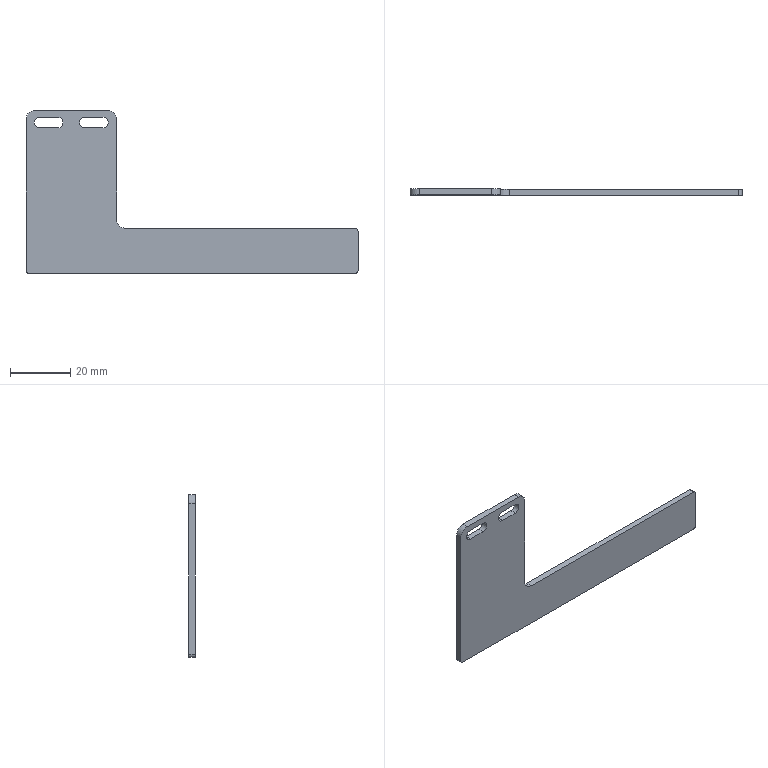Part | NX | features BREP 1 | 1 solid | 22 faces | box 110 x 2 x 54 mm | volume 5512 mm3 | plane 12 | cylinder 10 | commonest cylinder face diameters 3.5 x4 2 x3 6 x3
STEP:
#1=CARTESIAN_POINT('',(-55.,-2.,1.));
#2=VERTEX_POINT('',#1);
#3=CARTESIAN_POINT('',(-54.,-2.,0.));
#4=VERTEX_POINT('',#3);
#5=CARTESIAN_POINT('',(-54.,-2.,1.));
#6=DIRECTION('',(0.,-1.,0.));
#7=DIRECTION('',(-1.,0.,0.));
#8=AXIS2_PLACEMENT_3D('',#5,#6,#7);
#9=CIRCLE('',#8,1.);
#10=EDGE_CURVE('',#2,#4,#9,.T.);
#11=ORIENTED_EDGE('',*,*,#10,.F.);
#12=CARTESIAN_POINT('',(-55.,0.,1.));
#13=VERTEX_POINT('',#12);
#14=CARTESIAN_POINT('',(-55.,-2.,1.));
#15=DIRECTION('',(0.,-1.,0.));
#16=VECTOR('',#15,1000.);
#17=LINE('',#14,#16);
#18=EDGE_CURVE('',#13,#2,#17,.T.);
#19=ORIENTED_EDGE('',*,*,#18,.F.);
#20=CARTESIAN_POINT('',(-54.,0.,0.));
#21=VERTEX_POINT('',#20);
#22=CARTESIAN_POINT('',(-54.,0.,1.));
#23=DIRECTION('',(0.,1.,0.));
#24=DIRECTION('',(-1.,0.,0.));
#25=AXIS2_PLACEMENT_3D('',#22,#23,#24);
#26=CIRCLE('',#25,1.);
#27=EDGE_CURVE('',#21,#13,#26,.T.);
#28=ORIENTED_EDGE('',*,*,#27,.F.);
#29=CARTESIAN_POINT('',(-54.,0.,0.));
#30=DIRECTION('',(0.,1.,0.));
#31=VECTOR('',#30,1000.);
#32=LINE('',#29,#31);
#33=EDGE_CURVE('',#4,#21,#32,.T.);
#34=ORIENTED_EDGE('',*,*,#33,.F.);
#35=EDGE_LOOP('',(#11,#19,#28,#34));
#36=FACE_BOUND('',#35,.T.);
#37=CARTESIAN_POINT('',(-54.,0.,1.));
#38=DIRECTION('',(0.,1.,0.));
#39=DIRECTION('',(0.,0.,1.));
#40=AXIS2_PLACEMENT_3D('',#37,#38,#39);
#41=CYLINDRICAL_SURFACE('',#40,1.);
#42=ADVANCED_FACE('',(#36),#41,.T.);
#43=CARTESIAN_POINT('',(55.,0.,1.));
#44=VERTEX_POINT('',#43);
#45=CARTESIAN_POINT('',(54.,0.,0.));
#46=VERTEX_POINT('',#45);
#47=CARTESIAN_POINT('',(54.,0.,1.));
#48=DIRECTION('',(0.,1.,0.));
#49=DIRECTION('',(-1.,0.,0.));
#50=AXIS2_PLACEMENT_3D('',#47,#48,#49);
#51=CIRCLE('',#50,1.);
#52=EDGE_CURVE('',#44,#46,#51,.T.);
#53=ORIENTED_EDGE('',*,*,#52,.F.);
#54=CARTESIAN_POINT('',(55.,-2.,1.));
#55=VERTEX_POINT('',#54);
#56=CARTESIAN_POINT('',(55.,0.,1.));
#57=DIRECTION('',(0.,1.,0.));
#58=VECTOR('',#57,1000.);
#59=LINE('',#56,#58);
#60=EDGE_CURVE('',#55,#44,#59,.T.);
#61=ORIENTED_EDGE('',*,*,#60,.F.);
#62=CARTESIAN_POINT('',(54.,-2.,0.));
#63=VERTEX_POINT('',#62);
#64=CARTESIAN_POINT('',(54.,-2.,1.));
#65=DIRECTION('',(0.,-1.,0.));
#66=DIRECTION('',(-1.,0.,0.));
#67=AXIS2_PLACEMENT_3D('',#64,#65,#66);
#68=CIRCLE('',#67,1.);
#69=EDGE_CURVE('',#63,#55,#68,.T.);
#70=ORIENTED_EDGE('',*,*,#69,.F.);
#71=CARTESIAN_POINT('',(54.,0.,0.));
#72=DIRECTION('',(0.,-1.,0.));
#73=VECTOR('',#72,1000.);
#74=LINE('',#71,#73);
#75=EDGE_CURVE('',#46,#63,#74,.T.);
#76=ORIENTED_EDGE('',*,*,#75,.F.);
#77=EDGE_LOOP('',(#53,#61,#70,#76));
#78=FACE_BOUND('',#77,.T.);
#79=CARTESIAN_POINT('',(54.,0.,1.));
#80=DIRECTION('',(0.,-1.,0.));
#81=DIRECTION('',(0.,0.,-1.));
#82=AXIS2_PLACEMENT_3D('',#79,#80,#81);
#83=CYLINDRICAL_SURFACE('',#82,1.);
#84=ADVANCED_FACE('',(#78),#83,.T.);
#85=CARTESIAN_POINT('',(55.,-2.,14.));
#86=VERTEX_POINT('',#85);
#87=CARTESIAN_POINT('',(54.,-2.,15.));
#88=VERTEX_POINT('',#87);
#89=CARTESIAN_POINT('',(54.,-2.,14.));
#90=DIRECTION('',(0.,-1.,0.));
#91=DIRECTION('',(-1.,0.,0.));
#92=AXIS2_PLACEMENT_3D('',#89,#90,#91);
#93=CIRCLE('',#92,1.);
#94=EDGE_CURVE('',#86,#88,#93,.T.);
#95=ORIENTED_EDGE('',*,*,#94,.F.);
#96=CARTESIAN_POINT('',(55.,0.,14.));
#97=VERTEX_POINT('',#96);
#98=CARTESIAN_POINT('',(55.,-2.,14.));
#99=DIRECTION('',(0.,-1.,0.));
#100=VECTOR('',#99,1000.);
#101=LINE('',#98,#100);
#102=EDGE_CURVE('',#97,#86,#101,.T.);
#103=ORIENTED_EDGE('',*,*,#102,.F.);
#104=CARTESIAN_POINT('',(54.,0.,15.));
#105=VERTEX_POINT('',#104);
#106=CARTESIAN_POINT('',(54.,0.,14.));
#107=DIRECTION('',(0.,1.,0.));
#108=DIRECTION('',(-1.,0.,0.));
#109=AXIS2_PLACEMENT_3D('',#106,#107,#108);
#110=CIRCLE('',#109,1.);
#111=EDGE_CURVE('',#105,#97,#110,.T.);
#112=ORIENTED_EDGE('',*,*,#111,.F.);
#113=CARTESIAN_POINT('',(54.,0.,15.));
#114=DIRECTION('',(0.,1.,0.));
#115=VECTOR('',#114,1000.);
#116=LINE('',#113,#115);
#117=EDGE_CURVE('',#88,#105,#116,.T.);
#118=ORIENTED_EDGE('',*,*,#117,.F.);
#119=EDGE_LOOP('',(#95,#103,#112,#118));
#120=FACE_BOUND('',#119,.T.);
#121=CARTESIAN_POINT('',(54.,-10.,14.));
#122=DIRECTION('',(0.,-1.,0.));
#123=DIRECTION('',(0.,0.,-1.));
#124=AXIS2_PLACEMENT_3D('',#121,#122,#123);
#125=CYLINDRICAL_SURFACE('',#124,1.);
#126=ADVANCED_FACE('',(#120),#125,.T.);
#127=CARTESIAN_POINT('',(-22.,-2.,15.));
#128=VERTEX_POINT('',#127);
#129=CARTESIAN_POINT('',(-25.,-2.,18.));
#130=VERTEX_POINT('',#129);
#131=CARTESIAN_POINT('',(-22.,-2.,18.));
#132=DIRECTION('',(0.,1.,0.));
#133=DIRECTION('',(-1.,0.,0.));
#134=AXIS2_PLACEMENT_3D('',#131,#132,#133);
#135=CIRCLE('',#134,3.);
#136=EDGE_CURVE('',#128,#130,#135,.T.);
#137=ORIENTED_EDGE('',*,*,#136,.F.);
#138=CARTESIAN_POINT('',(-22.,0.,15.));
#139=VERTEX_POINT('',#138);
#140=CARTESIAN_POINT('',(-22.,-2.,15.));
#141=DIRECTION('',(0.,-1.,0.));
#142=VECTOR('',#141,1000.);
#143=LINE('',#140,#142);
#144=EDGE_CURVE('',#139,#128,#143,.T.);
#145=ORIENTED_EDGE('',*,*,#144,.F.);
#146=CARTESIAN_POINT('',(-25.,0.,18.));
#147=VERTEX_POINT('',#146);
#148=CARTESIAN_POINT('',(-22.,0.,18.));
#149=DIRECTION('',(0.,-1.,0.));
#150=DIRECTION('',(-1.,0.,0.));
#151=AXIS2_PLACEMENT_3D('',#148,#149,#150);
#152=CIRCLE('',#151,3.);
#153=EDGE_CURVE('',#147,#139,#152,.T.);
#154=ORIENTED_EDGE('',*,*,#153,.F.);
#155=CARTESIAN_POINT('',(-25.,0.,18.));
#156=DIRECTION('',(0.,1.,0.));
#157=VECTOR('',#156,1000.);
#158=LINE('',#155,#157);
#159=EDGE_CURVE('',#130,#147,#158,.T.);
#160=ORIENTED_EDGE('',*,*,#159,.F.);
#161=EDGE_LOOP('',(#137,#145,#154,#160));
#162=FACE_BOUND('',#161,.T.);
#163=CARTESIAN_POINT('',(-22.,-10.,18.));
#164=DIRECTION('',(0.,-1.,0.));
#165=DIRECTION('',(0.,0.,-1.));
#166=AXIS2_PLACEMENT_3D('',#163,#164,#165);
#167=CYLINDRICAL_SURFACE('',#166,3.);
#168=ADVANCED_FACE('',(#162),#167,.F.);
#169=CARTESIAN_POINT('',(-25.,-2.,51.));
#170=VERTEX_POINT('',#169);
#171=CARTESIAN_POINT('',(-28.,-2.,54.));
#172=VERTEX_POINT('',#171);
#173=CARTESIAN_POINT('',(-28.,-2.,51.));
#174=DIRECTION('',(0.,-1.,0.));
#175=DIRECTION('',(-1.,0.,0.));
#176=AXIS2_PLACEMENT_3D('',#173,#174,#175);
#177=CIRCLE('',#176,3.);
#178=EDGE_CURVE('',#170,#172,#177,.T.);
#179=ORIENTED_EDGE('',*,*,#178,.F.);
#180=CARTESIAN_POINT('',(-25.,0.,51.));
#181=VERTEX_POINT('',#180);
#182=CARTESIAN_POINT('',(-25.,-10.,51.));
#183=DIRECTION('',(0.,-1.,0.));
#184=VECTOR('',#183,1000.);
#185=LINE('',#182,#184);
#186=EDGE_CURVE('',#181,#170,#185,.T.);
#187=ORIENTED_EDGE('',*,*,#186,.F.);
#188=CARTESIAN_POINT('',(-28.,0.,54.));
#189=VERTEX_POINT('',#188);
#190=CARTESIAN_POINT('',(-28.,0.,51.));
#191=DIRECTION('',(0.,1.,0.));
#192=DIRECTION('',(-1.,0.,0.));
#193=AXIS2_PLACEMENT_3D('',#190,#191,#192);
#194=CIRCLE('',#193,3.);
#195=EDGE_CURVE('',#189,#181,#194,.T.);
#196=ORIENTED_EDGE('',*,*,#195,.F.);
#197=CARTESIAN_POINT('',(-28.,0.,54.));
#198=DIRECTION('',(0.,1.,0.));
#199=VECTOR('',#198,1000.);
#200=LINE('',#197,#199);
#201=EDGE_CURVE('',#172,#189,#200,.T.);
#202=ORIENTED_EDGE('',*,*,#201,.F.);
#203=EDGE_LOOP('',(#179,#187,#196,#202));
#204=FACE_BOUND('',#203,.T.);
#205=CARTESIAN_POINT('',(-28.,0.,51.));
#206=DIRECTION('',(0.,1.,0.));
#207=DIRECTION('',(0.,0.,1.));
#208=AXIS2_PLACEMENT_3D('',#205,#206,#207);
#209=CYLINDRICAL_SURFACE('',#208,3.);
#210=ADVANCED_FACE('',(#204),#209,.T.);
#211=CARTESIAN_POINT('',(-52.,-2.,54.));
#212=VERTEX_POINT('',#211);
#213=CARTESIAN_POINT('',(-55.,-2.,51.));
#214=VERTEX_POINT('',#213);
#215=CARTESIAN_POINT('',(-52.,-2.,51.));
#216=DIRECTION('',(0.,-1.,0.));
#217=DIRECTION('',(-1.,0.,0.));
#218=AXIS2_PLACEMENT_3D('',#215,#216,#217);
#219=CIRCLE('',#218,3.);
#220=EDGE_CURVE('',#212,#214,#219,.T.);
#221=ORIENTED_EDGE('',*,*,#220,.F.);
#222=CARTESIAN_POINT('',(-52.,0.,54.));
#223=VERTEX_POINT('',#222);
#224=CARTESIAN_POINT('',(-52.,-2.,54.));
#225=DIRECTION('',(0.,-1.,0.));
#226=VECTOR('',#225,1000.);
#227=LINE('',#224,#226);
#228=EDGE_CURVE('',#223,#212,#227,.T.);
#229=ORIENTED_EDGE('',*,*,#228,.F.);
#230=CARTESIAN_POINT('',(-55.,0.,51.));
#231=VERTEX_POINT('',#230);
#232=CARTESIAN_POINT('',(-52.,0.,51.));
#233=DIRECTION('',(0.,1.,0.));
#234=DIRECTION('',(-1.,0.,0.));
#235=AXIS2_PLACEMENT_3D('',#232,#233,#234);
#236=CIRCLE('',#235,3.);
#237=EDGE_CURVE('',#231,#223,#236,.T.);
#238=ORIENTED_EDGE('',*,*,#237,.F.);
#239=CARTESIAN_POINT('',(-55.,0.,51.));
#240=DIRECTION('',(0.,1.,0.));
#241=VECTOR('',#240,1000.);
#242=LINE('',#239,#241);
#243=EDGE_CURVE('',#214,#231,#242,.T.);
#244=ORIENTED_EDGE('',*,*,#243,.F.);
#245=EDGE_LOOP('',(#221,#229,#238,#244));
#246=FACE_BOUND('',#245,.T.);
#247=CARTESIAN_POINT('',(-52.,-2.,51.));
#248=DIRECTION('',(0.,-1.,0.));
#249=DIRECTION('',(0.,0.,-1.));
#250=AXIS2_PLACEMENT_3D('',#247,#248,#249);
#251=CYLINDRICAL_SURFACE('',#250,3.);
#252=ADVANCED_FACE('',(#246),#251,.T.);
#253=CARTESIAN_POINT('',(-35.5,-2.,51.75));
#254=VERTEX_POINT('',#253);
#255=CARTESIAN_POINT('',(-35.5,0.,51.75));
#256=VERTEX_POINT('',#255);
#257=CARTESIAN_POINT('',(-35.5,-10.,51.75));
#258=DIRECTION('',(0.,1.,0.));
#259=VECTOR('',#258,1000.);
#260=LINE('',#257,#259);
#261=EDGE_CURVE('',#254,#256,#260,.T.);
#262=ORIENTED_EDGE('',*,*,#261,.T.);
#263=CARTESIAN_POINT('',(-29.5,0.,51.75));
#264=VERTEX_POINT('',#263);
#265=CARTESIAN_POINT('',(-35.5,0.,51.75));
#266=DIRECTION('',(1.,0.,0.));
#267=VECTOR('',#266,1000.);
#268=LINE('',#265,#267);
#269=EDGE_CURVE('',#256,#264,#268,.T.);
#270=ORIENTED_EDGE('',*,*,#269,.T.);
#271=CARTESIAN_POINT('',(-29.5,-2.,51.75));
#272=VERTEX_POINT('',#271);
#273=CARTESIAN_POINT('',(-29.5,-10.,51.75));
#274=DIRECTION('',(0.,1.,0.));
#275=VECTOR('',#274,1000.);
#276=LINE('',#273,#275);
#277=EDGE_CURVE('',#272,#264,#276,.T.);
#278=ORIENTED_EDGE('',*,*,#277,.F.);
#279=CARTESIAN_POINT('',(-55.,-2.,51.75));
#280=DIRECTION('',(1.,0.,0.));
#281=VECTOR('',#280,1000.);
#282=LINE('',#279,#281);
#283=EDGE_CURVE('',#254,#272,#282,.T.);
#284=ORIENTED_EDGE('',*,*,#283,.F.);
#285=EDGE_LOOP('',(#262,#270,#278,#284));
#286=FACE_BOUND('',#285,.T.);
#287=CARTESIAN_POINT('',(-35.5,-10.,51.75));
#288=DIRECTION('',(0.,0.,1.));
#289=DIRECTION('',(1.,0.,0.));
#290=AXIS2_PLACEMENT_3D('',#287,#288,#289);
#291=PLANE('',#290);
#292=ADVANCED_FACE('',(#286),#291,.F.);
#293=ORIENTED_EDGE('',*,*,#277,.T.);
#294=CARTESIAN_POINT('',(-29.5,0.,48.25));
#295=VERTEX_POINT('',#294);
#296=CARTESIAN_POINT('',(-29.5,0.,50.));
#297=DIRECTION('',(0.,1.,0.));
#298=DIRECTION('',(0.,0.,1.));
#299=AXIS2_PLACEMENT_3D('',#296,#297,#298);
#300=CIRCLE('',#299,1.75);
#301=EDGE_CURVE('',#264,#295,#300,.T.);
#302=ORIENTED_EDGE('',*,*,#301,.T.);
#303=CARTESIAN_POINT('',(-29.5,-2.,48.25));
#304=VERTEX_POINT('',#303);
#305=CARTESIAN_POINT('',(-29.5,-10.,48.25));
#306=DIRECTION('',(0.,1.,0.));
#307=VECTOR('',#306,1000.);
#308=LINE('',#305,#307);
#309=EDGE_CURVE('',#304,#295,#308,.T.);
#310=ORIENTED_EDGE('',*,*,#309,.F.);
#311=CARTESIAN_POINT('',(-29.5,-2.,50.));
#312=DIRECTION('',(0.,1.,0.));
#313=DIRECTION('',(-1.,0.,0.));
#314=AXIS2_PLACEMENT_3D('',#311,#312,#313);
#315=CIRCLE('',#314,1.75);
#316=EDGE_CURVE('',#272,#304,#315,.T.);
#317=ORIENTED_EDGE('',*,*,#316,.F.);
#318=EDGE_LOOP('',(#293,#302,#310,#317));
#319=FACE_BOUND('',#318,.T.);
#320=CARTESIAN_POINT('',(-29.5,-10.,50.));
#321=DIRECTION('',(0.,1.,0.));
#322=DIRECTION('',(0.,0.,1.));
#323=AXIS2_PLACEMENT_3D('',#320,#321,#322);
#324=CYLINDRICAL_SURFACE('',#323,1.75);
#325=ADVANCED_FACE('',(#319),#324,.F.);
#326=ORIENTED_EDGE('',*,*,#309,.T.);
#327=CARTESIAN_POINT('',(-35.5,0.,48.25));
#328=VERTEX_POINT('',#327);
#329=CARTESIAN_POINT('',(-35.5,0.,48.25));
#330=DIRECTION('',(-1.,0.,0.));
#331=VECTOR('',#330,1000.);
#332=LINE('',#329,#331);
#333=EDGE_CURVE('',#295,#328,#332,.T.);
#334=ORIENTED_EDGE('',*,*,#333,.T.);
#335=CARTESIAN_POINT('',(-35.5,-2.,48.25));
#336=VERTEX_POINT('',#335);
#337=CARTESIAN_POINT('',(-35.5,-10.,48.25));
#338=DIRECTION('',(0.,1.,0.));
#339=VECTOR('',#338,1000.);
#340=LINE('',#337,#339);
#341=EDGE_CURVE('',#336,#328,#340,.T.);
#342=ORIENTED_EDGE('',*,*,#341,.F.);
#343=CARTESIAN_POINT('',(-55.,-2.,48.25));
#344=DIRECTION('',(-1.,0.,0.));
#345=VECTOR('',#344,1000.);
#346=LINE('',#343,#345);
#347=EDGE_CURVE('',#304,#336,#346,.T.);
#348=ORIENTED_EDGE('',*,*,#347,.F.);
#349=EDGE_LOOP('',(#326,#334,#342,#348));
#350=FACE_BOUND('',#349,.T.);
#351=CARTESIAN_POINT('',(-35.5,-10.,48.25));
#352=DIRECTION('',(0.,0.,-1.));
#353=DIRECTION('',(-1.,0.,0.));
#354=AXIS2_PLACEMENT_3D('',#351,#352,#353);
#355=PLANE('',#354);
#356=ADVANCED_FACE('',(#350),#355,.F.);
#357=ORIENTED_EDGE('',*,*,#341,.T.);
#358=CARTESIAN_POINT('',(-35.5,0.,50.));
#359=DIRECTION('',(0.,1.,0.));
#360=DIRECTION('',(0.,0.,1.));
#361=AXIS2_PLACEMENT_3D('',#358,#359,#360);
#362=CIRCLE('',#361,1.75);
#363=EDGE_CURVE('',#328,#256,#362,.T.);
#364=ORIENTED_EDGE('',*,*,#363,.T.);
#365=ORIENTED_EDGE('',*,*,#261,.F.);
#366=CARTESIAN_POINT('',(-35.5,-2.,50.));
#367=DIRECTION('',(0.,1.,0.));
#368=DIRECTION('',(-1.,0.,0.));
#369=AXIS2_PLACEMENT_3D('',#366,#367,#368);
#370=CIRCLE('',#369,1.75);
#371=EDGE_CURVE('',#336,#254,#370,.T.);
#372=ORIENTED_EDGE('',*,*,#371,.F.);
#373=EDGE_LOOP('',(#357,#364,#365,#372));
#374=FACE_BOUND('',#373,.T.);
#375=CARTESIAN_POINT('',(-35.5,-10.,50.));
#376=DIRECTION('',(0.,1.,0.));
#377=DIRECTION('',(0.,0.,1.));
#378=AXIS2_PLACEMENT_3D('',#375,#376,#377);
#379=CYLINDRICAL_SURFACE('',#378,1.75);
#380=ADVANCED_FACE('',(#374),#379,.F.);
#381=CARTESIAN_POINT('',(-50.5,-2.,51.75));
#382=VERTEX_POINT('',#381);
#383=CARTESIAN_POINT('',(-50.5,0.,51.75));
#384=VERTEX_POINT('',#383);
#385=CARTESIAN_POINT('',(-50.5,-10.,51.75));
#386=DIRECTION('',(0.,1.,0.));
#387=VECTOR('',#386,1000.);
#388=LINE('',#385,#387);
#389=EDGE_CURVE('',#382,#384,#388,.T.);
#390=ORIENTED_EDGE('',*,*,#389,.T.);
#391=CARTESIAN_POINT('',(-44.5,0.,51.75));
#392=VERTEX_POINT('',#391);
#393=CARTESIAN_POINT('',(-50.5,0.,51.75));
#394=DIRECTION('',(1.,0.,0.));
#395=VECTOR('',#394,1000.);
#396=LINE('',#393,#395);
#397=EDGE_CURVE('',#384,#392,#396,.T.);
#398=ORIENTED_EDGE('',*,*,#397,.T.);
#399=CARTESIAN_POINT('',(-44.5,-2.,51.75));
#400=VERTEX_POINT('',#399);
#401=CARTESIAN_POINT('',(-44.5,-10.,51.75));
#402=DIRECTION('',(0.,1.,0.));
#403=VECTOR('',#402,1000.);
#404=LINE('',#401,#403);
#405=EDGE_CURVE('',#400,#392,#404,.T.);
#406=ORIENTED_EDGE('',*,*,#405,.F.);
#407=CARTESIAN_POINT('',(-55.,-2.,51.75));
#408=DIRECTION('',(1.,0.,0.));
#409=VECTOR('',#408,1000.);
#410=LINE('',#407,#409);
#411=EDGE_CURVE('',#382,#400,#410,.T.);
#412=ORIENTED_EDGE('',*,*,#411,.F.);
#413=EDGE_LOOP('',(#390,#398,#406,#412));
#414=FACE_BOUND('',#413,.T.);
#415=CARTESIAN_POINT('',(-50.5,-10.,51.75));
#416=DIRECTION('',(0.,0.,1.));
#417=DIRECTION('',(1.,0.,0.));
#418=AXIS2_PLACEMENT_3D('',#415,#416,#417);
#419=PLANE('',#418);
#420=ADVANCED_FACE('',(#414),#419,.F.);
#421=ORIENTED_EDGE('',*,*,#405,.T.);
#422=CARTESIAN_POINT('',(-44.5,0.,48.25));
#423=VERTEX_POINT('',#422);
#424=CARTESIAN_POINT('',(-44.5,0.,50.));
#425=DIRECTION('',(0.,1.,0.));
#426=DIRECTION('',(0.,0.,1.));
#427=AXIS2_PLACEMENT_3D('',#424,#425,#426);
#428=CIRCLE('',#427,1.75);
#429=EDGE_CURVE('',#392,#423,#428,.T.);
#430=ORIENTED_EDGE('',*,*,#429,.T.);
#431=CARTESIAN_POINT('',(-44.5,-2.,48.25));
#432=VERTEX_POINT('',#431);
#433=CARTESIAN_POINT('',(-44.5,-10.,48.25));
#434=DIRECTION('',(0.,1.,0.));
#435=VECTOR('',#434,1000.);
#436=LINE('',#433,#435);
#437=EDGE_CURVE('',#432,#423,#436,.T.);
#438=ORIENTED_EDGE('',*,*,#437,.F.);
#439=CARTESIAN_POINT('',(-44.5,-2.,50.));
#440=DIRECTION('',(0.,1.,0.));
#441=DIRECTION('',(-1.,0.,0.));
#442=AXIS2_PLACEMENT_3D('',#439,#440,#441);
#443=CIRCLE('',#442,1.75);
#444=EDGE_CURVE('',#400,#432,#443,.T.);
#445=ORIENTED_EDGE('',*,*,#444,.F.);
#446=EDGE_LOOP('',(#421,#430,#438,#445));
#447=FACE_BOUND('',#446,.T.);
#448=CARTESIAN_POINT('',(-44.5,-10.,50.));
#449=DIRECTION('',(0.,1.,0.));
#450=DIRECTION('',(0.,0.,1.));
#451=AXIS2_PLACEMENT_3D('',#448,#449,#450);
#452=CYLINDRICAL_SURFACE('',#451,1.75);
#453=ADVANCED_FACE('',(#447),#452,.F.);
#454=ORIENTED_EDGE('',*,*,#437,.T.);
#455=CARTESIAN_POINT('',(-50.5,0.,48.25));
#456=VERTEX_POINT('',#455);
#457=CARTESIAN_POINT('',(-50.5,0.,48.25));
#458=DIRECTION('',(-1.,0.,0.));
#459=VECTOR('',#458,1000.);
#460=LINE('',#457,#459);
#461=EDGE_CURVE('',#423,#456,#460,.T.);
#462=ORIENTED_EDGE('',*,*,#461,.T.);
#463=CARTESIAN_POINT('',(-50.5,-2.,48.25));
#464=VERTEX_POINT('',#463);
#465=CARTESIAN_POINT('',(-50.5,-10.,48.25));
#466=DIRECTION('',(0.,1.,0.));
#467=VECTOR('',#466,1000.);
#468=LINE('',#465,#467);
#469=EDGE_CURVE('',#464,#456,#468,.T.);
#470=ORIENTED_EDGE('',*,*,#469,.F.);
#471=CARTESIAN_POINT('',(-55.,-2.,48.25));
#472=DIRECTION('',(-1.,0.,0.));
#473=VECTOR('',#472,1000.);
#474=LINE('',#471,#473);
#475=EDGE_CURVE('',#432,#464,#474,.T.);
#476=ORIENTED_EDGE('',*,*,#475,.F.);
#477=EDGE_LOOP('',(#454,#462,#470,#476));
#478=FACE_BOUND('',#477,.T.);
#479=CARTESIAN_POINT('',(-50.5,-10.,48.25));
#480=DIRECTION('',(0.,0.,-1.));
#481=DIRECTION('',(-1.,0.,0.));
#482=AXIS2_PLACEMENT_3D('',#479,#480,#481);
#483=PLANE('',#482);
#484=ADVANCED_FACE('',(#478),#483,.F.);
#485=ORIENTED_EDGE('',*,*,#469,.T.);
#486=CARTESIAN_POINT('',(-50.5,0.,50.));
#487=DIRECTION('',(0.,1.,0.));
#488=DIRECTION('',(0.,0.,1.));
#489=AXIS2_PLACEMENT_3D('',#486,#487,#488);
#490=CIRCLE('',#489,1.75);
#491=EDGE_CURVE('',#456,#384,#490,.T.);
#492=ORIENTED_EDGE('',*,*,#491,.T.);
#493=ORIENTED_EDGE('',*,*,#389,.F.);
#494=CARTESIAN_POINT('',(-50.5,-2.,50.));
#495=DIRECTION('',(0.,1.,0.));
#496=DIRECTION('',(-1.,0.,0.));
#497=AXIS2_PLACEMENT_3D('',#494,#495,#496);
#498=CIRCLE('',#497,1.75);
#499=EDGE_CURVE('',#464,#382,#498,.T.);
#500=ORIENTED_EDGE('',*,*,#499,.F.);
#501=EDGE_LOOP('',(#485,#492,#493,#500));
#502=FACE_BOUND('',#501,.T.);
#503=CARTESIAN_POINT('',(-50.5,-10.,50.));
#504=DIRECTION('',(0.,1.,0.));
#505=DIRECTION('',(0.,0.,1.));
#506=AXIS2_PLACEMENT_3D('',#503,#504,#505);
#507=CYLINDRICAL_SURFACE('',#506,1.75);
#508=ADVANCED_FACE('',(#502),#507,.F.);
#509=CARTESIAN_POINT('',(-25.,0.,93.));
#510=DIRECTION('',(0.,0.,1.));
#511=VECTOR('',#510,1000.);
#512=LINE('',#509,#511);
#513=EDGE_CURVE('',#147,#181,#512,.T.);
#514=ORIENTED_EDGE('',*,*,#513,.T.);
#515=ORIENTED_EDGE('',*,*,#186,.T.);
#516=CARTESIAN_POINT('',(-25.,-2.,54.));
#517=DIRECTION('',(0.,0.,1.));
#518=VECTOR('',#517,1000.);
#519=LINE('',#516,#518);
#520=EDGE_CURVE('',#130,#170,#519,.T.);
#521=ORIENTED_EDGE('',*,*,#520,.F.);
#522=ORIENTED_EDGE('',*,*,#159,.T.);
#523=EDGE_LOOP('',(#514,#515,#521,#522));
#524=FACE_BOUND('',#523,.T.);
#525=CARTESIAN_POINT('',(-25.,-10.,93.));
#526=DIRECTION('',(-1.,0.,0.));
#527=DIRECTION('',(0.,0.,1.));
#528=AXIS2_PLACEMENT_3D('',#525,#526,#527);
#529=PLANE('',#528);
#530=ADVANCED_FACE('',(#524),#529,.F.);
#531=CARTESIAN_POINT('',(-55.,-2.,15.));
#532=DIRECTION('',(-1.,0.,0.));
#533=VECTOR('',#532,1000.);
#534=LINE('',#531,#533);
#535=EDGE_CURVE('',#88,#128,#534,.T.);
#536=ORIENTED_EDGE('',*,*,#535,.F.);
#537=ORIENTED_EDGE('',*,*,#117,.T.);
#538=CARTESIAN_POINT('',(135.,0.,15.));
#539=DIRECTION('',(-1.,0.,0.));
#540=VECTOR('',#539,1000.);
#541=LINE('',#538,#540);
#542=EDGE_CURVE('',#105,#139,#541,.T.);
#543=ORIENTED_EDGE('',*,*,#542,.T.);
#544=ORIENTED_EDGE('',*,*,#144,.T.);
#545=EDGE_LOOP('',(#536,#537,#543,#544));
#546=FACE_BOUND('',#545,.T.);
#547=CARTESIAN_POINT('',(135.,-10.,15.));
#548=DIRECTION('',(0.,0.,-1.));
#549=DIRECTION('',(-1.,0.,0.));
#550=AXIS2_PLACEMENT_3D('',#547,#548,#549);
#551=PLANE('',#550);
#552=ADVANCED_FACE('',(#546),#551,.F.);
#553=CARTESIAN_POINT('',(-55.,0.,0.));
#554=DIRECTION('',(1.,0.,0.));
#555=VECTOR('',#554,1000.);
#556=LINE('',#553,#555);
#557=EDGE_CURVE('',#21,#46,#556,.T.);
#558=ORIENTED_EDGE('',*,*,#557,.T.);
#559=ORIENTED_EDGE('',*,*,#75,.T.);
#560=CARTESIAN_POINT('',(-55.,-2.,0.));
#561=DIRECTION('',(1.,0.,0.));
#562=VECTOR('',#561,1000.);
#563=LINE('',#560,#562);
#564=EDGE_CURVE('',#4,#63,#563,.T.);
#565=ORIENTED_EDGE('',*,*,#564,.F.);
#566=ORIENTED_EDGE('',*,*,#33,.T.);
#567=EDGE_LOOP('',(#558,#559,#565,#566));
#568=FACE_BOUND('',#567,.T.);
#569=CARTESIAN_POINT('',(0.,0.,0.));
#570=DIRECTION('',(0.,0.,-1.));
#571=DIRECTION('',(-1.,0.,0.));
#572=AXIS2_PLACEMENT_3D('',#569,#570,#571);
#573=PLANE('',#572);
#574=ADVANCED_FACE('',(#568),#573,.T.);
#575=CARTESIAN_POINT('',(-55.,0.,54.));
#576=DIRECTION('',(1.,0.,0.));
#577=VECTOR('',#576,1000.);
#578=LINE('',#575,#577);
#579=EDGE_CURVE('',#223,#189,#578,.T.);
#580=ORIENTED_EDGE('',*,*,#579,.F.);
#581=ORIENTED_EDGE('',*,*,#228,.T.);
#582=CARTESIAN_POINT('',(-55.,-2.,54.));
#583=DIRECTION('',(1.,0.,0.));
#584=VECTOR('',#583,1000.);
#585=LINE('',#582,#584);
#586=EDGE_CURVE('',#212,#172,#585,.T.);
#587=ORIENTED_EDGE('',*,*,#586,.T.);
#588=ORIENTED_EDGE('',*,*,#201,.T.);
#589=EDGE_LOOP('',(#580,#581,#587,#588));
#590=FACE_BOUND('',#589,.T.);
#591=CARTESIAN_POINT('',(0.,0.,54.));
#592=DIRECTION('',(0.,0.,-1.));
#593=DIRECTION('',(-1.,0.,0.));
#594=AXIS2_PLACEMENT_3D('',#591,#592,#593);
#595=PLANE('',#594);
#596=ADVANCED_FACE('',(#590),#595,.F.);
#597=CARTESIAN_POINT('',(-55.,0.,54.));
#598=DIRECTION('',(0.,0.,-1.));
#599=VECTOR('',#598,1000.);
#600=LINE('',#597,#599);
#601=EDGE_CURVE('',#231,#13,#600,.T.);
#602=ORIENTED_EDGE('',*,*,#601,.T.);
#603=ORIENTED_EDGE('',*,*,#18,.T.);
#604=CARTESIAN_POINT('',(-55.,-2.,54.));
#605=DIRECTION('',(0.,0.,-1.));
#606=VECTOR('',#605,1000.);
#607=LINE('',#604,#606);
#608=EDGE_CURVE('',#214,#2,#607,.T.);
#609=ORIENTED_EDGE('',*,*,#608,.F.);
#610=ORIENTED_EDGE('',*,*,#243,.T.);
#611=EDGE_LOOP('',(#602,#603,#609,#610));
#612=FACE_BOUND('',#611,.T.);
#613=CARTESIAN_POINT('',(-55.,-2.,54.));
#614=DIRECTION('',(-1.,0.,0.));
#615=DIRECTION('',(0.,0.,1.));
#616=AXIS2_PLACEMENT_3D('',#613,#614,#615);
#617=PLANE('',#616);
#618=ADVANCED_FACE('',(#612),#617,.T.);
#619=ORIENTED_EDGE('',*,*,#542,.F.);
#620=ORIENTED_EDGE('',*,*,#111,.T.);
#621=CARTESIAN_POINT('',(55.,0.,54.));
#622=DIRECTION('',(0.,0.,-1.));
#623=VECTOR('',#622,1000.);
#624=LINE('',#621,#623);
#625=EDGE_CURVE('',#97,#44,#624,.T.);
#626=ORIENTED_EDGE('',*,*,#625,.T.);
#627=ORIENTED_EDGE('',*,*,#52,.T.);
#628=ORIENTED_EDGE('',*,*,#557,.F.);
#629=ORIENTED_EDGE('',*,*,#27,.T.);
#630=ORIENTED_EDGE('',*,*,#601,.F.);
#631=ORIENTED_EDGE('',*,*,#237,.T.);
#632=ORIENTED_EDGE('',*,*,#579,.T.);
#633=ORIENTED_EDGE('',*,*,#195,.T.);
#634=ORIENTED_EDGE('',*,*,#513,.F.);
#635=ORIENTED_EDGE('',*,*,#153,.T.);
#636=EDGE_LOOP('',(#619,#620,#626,#627,#628,#629,#630,#631,#632,#633,#634,#635));
#637=FACE_BOUND('',#636,.T.);
#638=ORIENTED_EDGE('',*,*,#491,.F.);
#639=ORIENTED_EDGE('',*,*,#461,.F.);
#640=ORIENTED_EDGE('',*,*,#429,.F.);
#641=ORIENTED_EDGE('',*,*,#397,.F.);
#642=EDGE_LOOP('',(#638,#639,#640,#641));
#643=FACE_BOUND('',#642,.T.);
#644=ORIENTED_EDGE('',*,*,#363,.F.);
#645=ORIENTED_EDGE('',*,*,#333,.F.);
#646=ORIENTED_EDGE('',*,*,#301,.F.);
#647=ORIENTED_EDGE('',*,*,#269,.F.);
#648=EDGE_LOOP('',(#644,#645,#646,#647));
#649=FACE_BOUND('',#648,.T.);
#650=CARTESIAN_POINT('',(-55.,0.,54.));
#651=DIRECTION('',(0.,1.,0.));
#652=DIRECTION('',(-1.,0.,0.));
#653=AXIS2_PLACEMENT_3D('',#650,#651,#652);
#654=PLANE('',#653);
#655=ADVANCED_FACE('',(#637,#643,#649),#654,.T.);
#656=ORIENTED_EDGE('',*,*,#625,.F.);
#657=ORIENTED_EDGE('',*,*,#102,.T.);
#658=CARTESIAN_POINT('',(55.,-2.,54.));
#659=DIRECTION('',(0.,0.,-1.));
#660=VECTOR('',#659,1000.);
#661=LINE('',#658,#660);
#662=EDGE_CURVE('',#86,#55,#661,.T.);
#663=ORIENTED_EDGE('',*,*,#662,.T.);
#664=ORIENTED_EDGE('',*,*,#60,.T.);
#665=EDGE_LOOP('',(#656,#657,#663,#664));
#666=FACE_BOUND('',#665,.T.);
#667=CARTESIAN_POINT('',(55.,0.,54.));
#668=DIRECTION('',(1.,0.,0.));
#669=DIRECTION('',(0.,0.,-1.));
#670=AXIS2_PLACEMENT_3D('',#667,#668,#669);
#671=PLANE('',#670);
#672=ADVANCED_FACE('',(#666),#671,.T.);
#673=ORIENTED_EDGE('',*,*,#662,.F.);
#674=ORIENTED_EDGE('',*,*,#94,.T.);
#675=ORIENTED_EDGE('',*,*,#535,.T.);
#676=ORIENTED_EDGE('',*,*,#136,.T.);
#677=ORIENTED_EDGE('',*,*,#520,.T.);
#678=ORIENTED_EDGE('',*,*,#178,.T.);
#679=ORIENTED_EDGE('',*,*,#586,.F.);
#680=ORIENTED_EDGE('',*,*,#220,.T.);
#681=ORIENTED_EDGE('',*,*,#608,.T.);
#682=ORIENTED_EDGE('',*,*,#10,.T.);
#683=ORIENTED_EDGE('',*,*,#564,.T.);
#684=ORIENTED_EDGE('',*,*,#69,.T.);
#685=EDGE_LOOP('',(#673,#674,#675,#676,#677,#678,#679,#680,#681,#682,#683,#684));
#686=FACE_BOUND('',#685,.T.);
#687=ORIENTED_EDGE('',*,*,#475,.T.);
#688=ORIENTED_EDGE('',*,*,#499,.T.);
#689=ORIENTED_EDGE('',*,*,#411,.T.);
#690=ORIENTED_EDGE('',*,*,#444,.T.);
#691=EDGE_LOOP('',(#687,#688,#689,#690));
#692=FACE_BOUND('',#691,.T.);
#693=ORIENTED_EDGE('',*,*,#347,.T.);
#694=ORIENTED_EDGE('',*,*,#371,.T.);
#695=ORIENTED_EDGE('',*,*,#283,.T.);
#696=ORIENTED_EDGE('',*,*,#316,.T.);
#697=EDGE_LOOP('',(#693,#694,#695,#696));
#698=FACE_BOUND('',#697,.T.);
#699=CARTESIAN_POINT('',(-55.,-2.,54.));
#700=DIRECTION('',(0.,1.,0.));
#701=DIRECTION('',(-1.,0.,0.));
#702=AXIS2_PLACEMENT_3D('',#699,#700,#701);
#703=PLANE('',#702);
#704=ADVANCED_FACE('',(#686,#692,#698),#703,.F.);
#705=CLOSED_SHELL('',(#42,#84,#126,#168,#210,#252,#292,#325,#356,#380,#420,#453,#484,#508,#530,#552,#574,#596,#618,#655,#672,#704));
#706=MANIFOLD_SOLID_BREP('',#705);
#707=(LENGTH_UNIT()NAMED_UNIT(*)SI_UNIT(.MILLI.,.METRE.));
#708=UNCERTAINTY_MEASURE_WITH_UNIT(LENGTH_MEASURE(0.00001),#707,'','');
#709=(NAMED_UNIT(*)PLANE_ANGLE_UNIT()SI_UNIT($,.RADIAN.));
#710=(NAMED_UNIT(*)SI_UNIT($,.STERADIAN.)SOLID_ANGLE_UNIT());
#711=(GEOMETRIC_REPRESENTATION_CONTEXT(3)GLOBAL_UNCERTAINTY_ASSIGNED_CONTEXT((#708))GLOBAL_UNIT_ASSIGNED_CONTEXT((#707,#709,#710))REPRESENTATION_CONTEXT('',''));
#712=ADVANCED_BREP_SHAPE_REPRESENTATION('',(#706),#711);